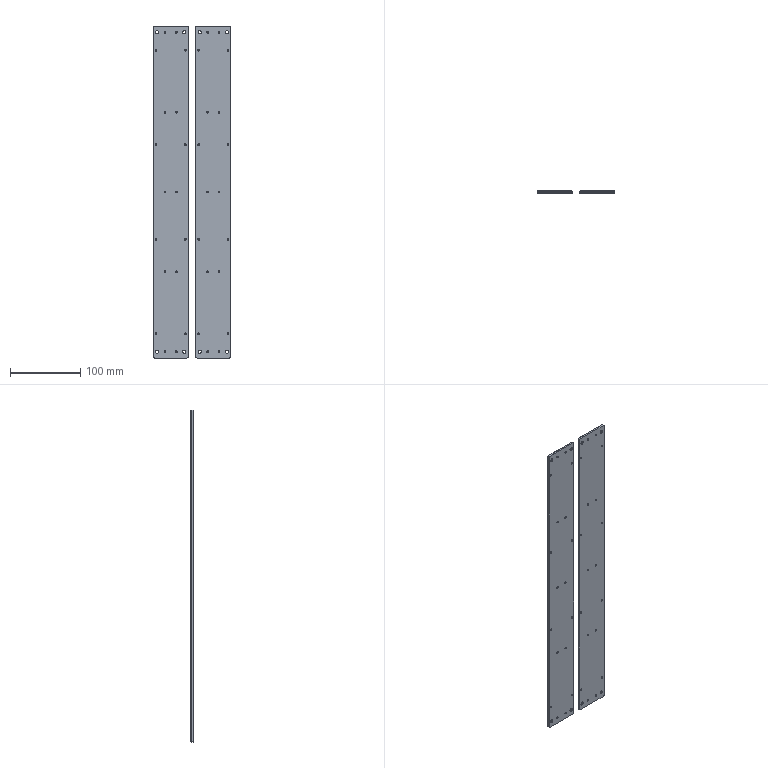CAM job | NX | 3+2 milling, drilling | part box 111 x 3 x 474 mm | stock box 116 x 3 x 479 mm
Tools:
number,name,description,diameter,corner_radius,flute_length,length,flutes
9,D10,平底铣刀-粗,10.0,0.0,35.0,75.0,2
17,D2-J,平底铣刀-精,2.0,0.0,50.0,75.0,2
11,D4-J,平底铣刀-精,4.0,0.0,50.0,75.0,2
7,D6-J,平底铣刀-精,6.0,0.0,25.0,75.0,2
2,D6倒角刀,倒角刀,6.0,0.0,3.0,25.0,2
12,ZT2.5,钻头,2.5,0.0,35.0,50.0,2
11,ZT4.5,钻头,4.5,0.0,35.0,50.0,2
Operations:
program,operation,operation_type,tool,method,geometry_group,spindle_rpm,surface_speed,feed_per_tooth,feed_cut,feed_plunge,cut_length_mm,path_length_mm,cut_time_min,machine_time_min
A,打点,Operation,D6倒角刀,METHOD,W-A,3000.0,56.549,0.0333,200.0,0.0,20.0,743.098,0.1,0.1723
A,打点_2,Operation,D6倒角刀,METHOD,W-A,3000.0,56.549,0.0333,200.0,0.0,72.0,1401.525,0.36,0.493
A,打孔,Operation,ZT2.5,METHOD,W-A,3800.0,29.845,0.0105,80.0,0.0,133.2,1523.925,1.665,1.804
A,打孔_2,Operation,ZT4.5,METHOD,W-A,2800.0,39.584,0.0214,120.0,0.0,29.6,762.298,0.2467,0.3199
A,外形粗_2,VolumeBased25DMillingOperation,D10,METHOD,W-A,6000.0,188.0,0.25,4000.0,80.0,15075.55,15278.751,3.769,3.789
A,等高螺旋爬面_COPY,ZLevelMilling,D4-J,等高爬面-切深K-步距G,W-A,7000.0,175.924,0.1786,2500.0,100.0,14612.923,15577.447,5.845,5.942
A,底壁铣螺旋精光-中_COPY,VolumeBased25DMillingOperation,D2-J,螺旋精光-切深K-步距G,W-A,8000.0,50.264,0.0375,600.0,100.0,466.122,1479.358,0.7769,0.8782
A,底壁铣螺旋精光-中_COPY_COPY,VolumeBased25DMillingOperation,D2-J,螺旋精光-切深K-步距G,W-A,8000.0,50.266,0.0125,200.0,100.0,1311.68,3983.207,6.558,6.826
A,钻倒角_1,Operation,D6倒角刀,METHOD,W-A,5000.0,94.248,0.015,150.0,0.0,171.0,1674.943,1.14,1.29
A,底壁铣倒角_COPY,VolumeBased25DMillingOperation,D6倒角刀,爬面_倒角-切深0-步距G,W-A,6500.0,122.519,0.1154,1500.0,100.0,2112.084,2452.066,1.408,1.442
A,外形半精_2,VolumeBased25DMillingOperation,D6-J,METHOD,W-A,6000.0,113.0,0.0833,1000.0,100.0,2136.748,2709.185,2.137,2.194
A,外形精_2,VolumeBased25DMillingOperation,D6-J,METHOD,W-A,6000.0,113.0,0.0833,1000.0,100.0,2136.348,2709.928,2.136,2.194